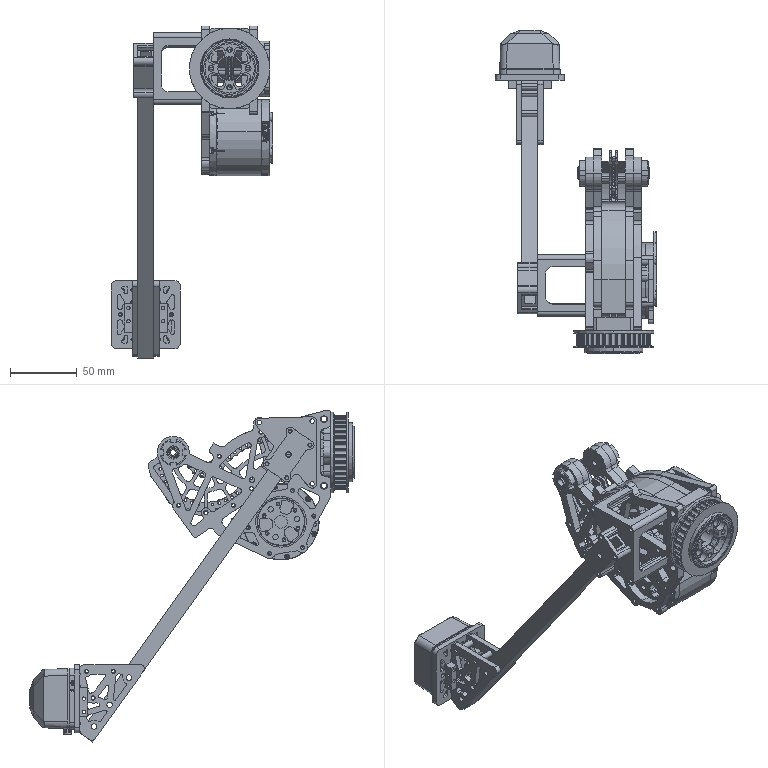Part | SolidWorks | 90 solids | 6848 faces | volume 313010 mm3 | cylinder 3327 | plane 2309 | spline 432 | torus 404 | cone 376 | commonest cylinder face diameters 2 x514 2.5 x373 5 x357 4 x273 2.05 x188 2.2 x132